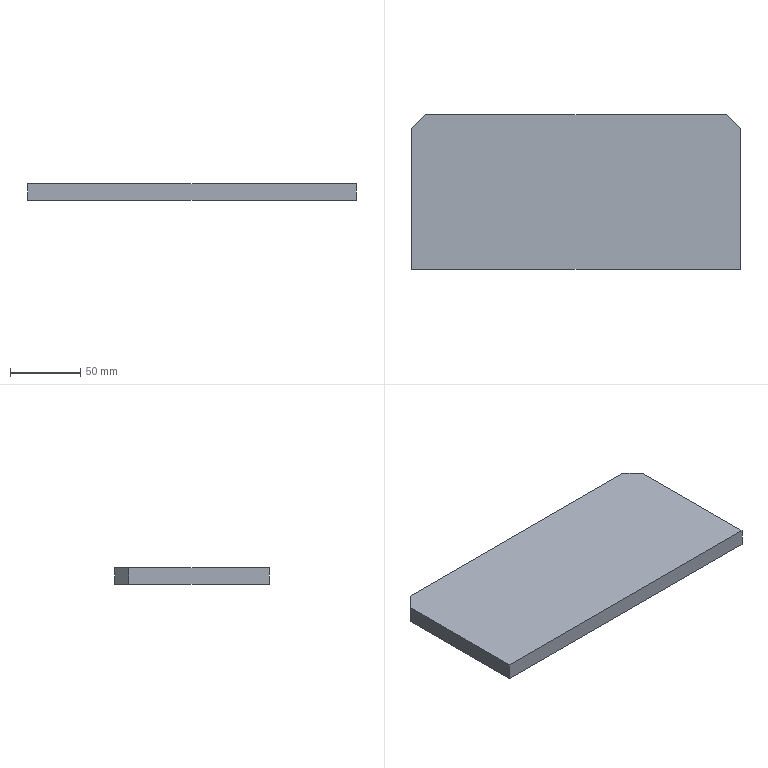Part | SolidWorks | features BaseBody 1 | 1 solid | 8 faces | box 234 x 110 x 12 mm | volume 307680 mm3 | plane 8
STEP:
#1=CARTESIAN_POINT('',(117.,-55.,0.));
#2=VERTEX_POINT('',#1);
#3=CARTESIAN_POINT('',(117.,45.,0.));
#4=VERTEX_POINT('',#3);
#5=CARTESIAN_POINT('',(117.,45.,0.));
#6=DIRECTION('',(0.,1.,0.));
#7=VECTOR('',#6,1000.);
#8=LINE('',#5,#7);
#9=EDGE_CURVE('',#2,#4,#8,.T.);
#10=ORIENTED_EDGE('',*,*,#9,.T.);
#11=CARTESIAN_POINT('',(117.,45.,12.));
#12=VERTEX_POINT('',#11);
#13=CARTESIAN_POINT('',(117.,45.,12.));
#14=DIRECTION('',(0.,0.,-1.));
#15=VECTOR('',#14,1000.);
#16=LINE('',#13,#15);
#17=EDGE_CURVE('',#12,#4,#16,.T.);
#18=ORIENTED_EDGE('',*,*,#17,.F.);
#19=CARTESIAN_POINT('',(117.,-55.,12.));
#20=VERTEX_POINT('',#19);
#21=CARTESIAN_POINT('',(117.,45.,12.));
#22=DIRECTION('',(0.,1.,0.));
#23=VECTOR('',#22,1000.);
#24=LINE('',#21,#23);
#25=EDGE_CURVE('',#20,#12,#24,.T.);
#26=ORIENTED_EDGE('',*,*,#25,.F.);
#27=CARTESIAN_POINT('',(117.,-55.,12.));
#28=DIRECTION('',(0.,0.,-1.));
#29=VECTOR('',#28,1000.);
#30=LINE('',#27,#29);
#31=EDGE_CURVE('',#20,#2,#30,.T.);
#32=ORIENTED_EDGE('',*,*,#31,.T.);
#33=EDGE_LOOP('',(#10,#18,#26,#32));
#34=FACE_OUTER_BOUND('',#33,.T.);
#35=CARTESIAN_POINT('',(117.,45.,12.));
#36=DIRECTION('',(-1.,0.,0.));
#37=DIRECTION('',(0.,0.,1.));
#38=AXIS2_PLACEMENT_3D('',#35,#36,#37);
#39=PLANE('',#38);
#40=ADVANCED_FACE('',(#34),#39,.F.);
#41=CARTESIAN_POINT('',(107.,55.,0.));
#42=VERTEX_POINT('',#41);
#43=CARTESIAN_POINT('',(107.,55.,0.));
#44=DIRECTION('',(-0.7071,0.7071,0.));
#45=VECTOR('',#44,1000.);
#46=LINE('',#43,#45);
#47=EDGE_CURVE('',#4,#42,#46,.T.);
#48=ORIENTED_EDGE('',*,*,#47,.T.);
#49=CARTESIAN_POINT('',(107.,55.,12.));
#50=VERTEX_POINT('',#49);
#51=CARTESIAN_POINT('',(107.,55.,12.));
#52=DIRECTION('',(0.,0.,-1.));
#53=VECTOR('',#52,1000.);
#54=LINE('',#51,#53);
#55=EDGE_CURVE('',#50,#42,#54,.T.);
#56=ORIENTED_EDGE('',*,*,#55,.F.);
#57=CARTESIAN_POINT('',(107.,55.,12.));
#58=DIRECTION('',(-0.7071,0.7071,0.));
#59=VECTOR('',#58,1000.);
#60=LINE('',#57,#59);
#61=EDGE_CURVE('',#12,#50,#60,.T.);
#62=ORIENTED_EDGE('',*,*,#61,.F.);
#63=ORIENTED_EDGE('',*,*,#17,.T.);
#64=EDGE_LOOP('',(#48,#56,#62,#63));
#65=FACE_OUTER_BOUND('',#64,.T.);
#66=CARTESIAN_POINT('',(107.,55.,12.));
#67=DIRECTION('',(-0.7071,-0.7071,0.));
#68=DIRECTION('',(0.7071,-0.7071,0.));
#69=AXIS2_PLACEMENT_3D('',#66,#67,#68);
#70=PLANE('',#69);
#71=ADVANCED_FACE('',(#65),#70,.F.);
#72=CARTESIAN_POINT('',(-107.,55.,0.));
#73=VERTEX_POINT('',#72);
#74=CARTESIAN_POINT('',(-107.,55.,0.));
#75=DIRECTION('',(-1.,0.,0.));
#76=VECTOR('',#75,1000.);
#77=LINE('',#74,#76);
#78=EDGE_CURVE('',#42,#73,#77,.T.);
#79=ORIENTED_EDGE('',*,*,#78,.T.);
#80=CARTESIAN_POINT('',(-107.,55.,12.));
#81=VERTEX_POINT('',#80);
#82=CARTESIAN_POINT('',(-107.,55.,12.));
#83=DIRECTION('',(0.,0.,-1.));
#84=VECTOR('',#83,1000.);
#85=LINE('',#82,#84);
#86=EDGE_CURVE('',#81,#73,#85,.T.);
#87=ORIENTED_EDGE('',*,*,#86,.F.);
#88=CARTESIAN_POINT('',(-107.,55.,12.));
#89=DIRECTION('',(-1.,0.,0.));
#90=VECTOR('',#89,1000.);
#91=LINE('',#88,#90);
#92=EDGE_CURVE('',#50,#81,#91,.T.);
#93=ORIENTED_EDGE('',*,*,#92,.F.);
#94=ORIENTED_EDGE('',*,*,#55,.T.);
#95=EDGE_LOOP('',(#79,#87,#93,#94));
#96=FACE_OUTER_BOUND('',#95,.T.);
#97=CARTESIAN_POINT('',(-107.,55.,12.));
#98=DIRECTION('',(0.,-1.,0.));
#99=DIRECTION('',(0.,0.,-1.));
#100=AXIS2_PLACEMENT_3D('',#97,#98,#99);
#101=PLANE('',#100);
#102=ADVANCED_FACE('',(#96),#101,.F.);
#103=CARTESIAN_POINT('',(-117.,45.,0.));
#104=VERTEX_POINT('',#103);
#105=CARTESIAN_POINT('',(-117.,45.,0.));
#106=DIRECTION('',(-0.7071,-0.7071,0.));
#107=VECTOR('',#106,1000.);
#108=LINE('',#105,#107);
#109=EDGE_CURVE('',#73,#104,#108,.T.);
#110=ORIENTED_EDGE('',*,*,#109,.T.);
#111=CARTESIAN_POINT('',(-117.,45.,12.));
#112=VERTEX_POINT('',#111);
#113=CARTESIAN_POINT('',(-117.,45.,12.));
#114=DIRECTION('',(0.,0.,-1.));
#115=VECTOR('',#114,1000.);
#116=LINE('',#113,#115);
#117=EDGE_CURVE('',#112,#104,#116,.T.);
#118=ORIENTED_EDGE('',*,*,#117,.F.);
#119=CARTESIAN_POINT('',(-117.,45.,12.));
#120=DIRECTION('',(-0.7071,-0.7071,0.));
#121=VECTOR('',#120,1000.);
#122=LINE('',#119,#121);
#123=EDGE_CURVE('',#81,#112,#122,.T.);
#124=ORIENTED_EDGE('',*,*,#123,.F.);
#125=ORIENTED_EDGE('',*,*,#86,.T.);
#126=EDGE_LOOP('',(#110,#118,#124,#125));
#127=FACE_OUTER_BOUND('',#126,.T.);
#128=CARTESIAN_POINT('',(-117.,45.,12.));
#129=DIRECTION('',(0.7071,-0.7071,0.));
#130=DIRECTION('',(0.7071,0.7071,0.));
#131=AXIS2_PLACEMENT_3D('',#128,#129,#130);
#132=PLANE('',#131);
#133=ADVANCED_FACE('',(#127),#132,.F.);
#134=CARTESIAN_POINT('',(-117.,-55.,0.));
#135=VERTEX_POINT('',#134);
#136=CARTESIAN_POINT('',(-117.,45.,0.));
#137=DIRECTION('',(0.,-1.,0.));
#138=VECTOR('',#137,1000.);
#139=LINE('',#136,#138);
#140=EDGE_CURVE('',#104,#135,#139,.T.);
#141=ORIENTED_EDGE('',*,*,#140,.T.);
#142=CARTESIAN_POINT('',(-117.,-55.,12.));
#143=VERTEX_POINT('',#142);
#144=CARTESIAN_POINT('',(-117.,-55.,12.));
#145=DIRECTION('',(0.,0.,-1.));
#146=VECTOR('',#145,1000.);
#147=LINE('',#144,#146);
#148=EDGE_CURVE('',#143,#135,#147,.T.);
#149=ORIENTED_EDGE('',*,*,#148,.F.);
#150=CARTESIAN_POINT('',(-117.,45.,12.));
#151=DIRECTION('',(0.,-1.,0.));
#152=VECTOR('',#151,1000.);
#153=LINE('',#150,#152);
#154=EDGE_CURVE('',#112,#143,#153,.T.);
#155=ORIENTED_EDGE('',*,*,#154,.F.);
#156=ORIENTED_EDGE('',*,*,#117,.T.);
#157=EDGE_LOOP('',(#141,#149,#155,#156));
#158=FACE_OUTER_BOUND('',#157,.T.);
#159=CARTESIAN_POINT('',(-117.,45.,12.));
#160=DIRECTION('',(1.,0.,0.));
#161=DIRECTION('',(0.,1.,0.));
#162=AXIS2_PLACEMENT_3D('',#159,#160,#161);
#163=PLANE('',#162);
#164=ADVANCED_FACE('',(#158),#163,.F.);
#165=CARTESIAN_POINT('',(-117.,-55.,0.));
#166=DIRECTION('',(1.,0.,0.));
#167=VECTOR('',#166,1000.);
#168=LINE('',#165,#167);
#169=EDGE_CURVE('',#135,#2,#168,.T.);
#170=ORIENTED_EDGE('',*,*,#169,.T.);
#171=ORIENTED_EDGE('',*,*,#31,.F.);
#172=CARTESIAN_POINT('',(-117.,-55.,12.));
#173=DIRECTION('',(1.,0.,0.));
#174=VECTOR('',#173,1000.);
#175=LINE('',#172,#174);
#176=EDGE_CURVE('',#143,#20,#175,.T.);
#177=ORIENTED_EDGE('',*,*,#176,.F.);
#178=ORIENTED_EDGE('',*,*,#148,.T.);
#179=EDGE_LOOP('',(#170,#171,#177,#178));
#180=FACE_OUTER_BOUND('',#179,.T.);
#181=CARTESIAN_POINT('',(-117.,-55.,12.));
#182=DIRECTION('',(0.,1.,0.));
#183=DIRECTION('',(0.,0.,1.));
#184=AXIS2_PLACEMENT_3D('',#181,#182,#183);
#185=PLANE('',#184);
#186=ADVANCED_FACE('',(#180),#185,.F.);
#187=ORIENTED_EDGE('',*,*,#25,.T.);
#188=ORIENTED_EDGE('',*,*,#61,.T.);
#189=ORIENTED_EDGE('',*,*,#92,.T.);
#190=ORIENTED_EDGE('',*,*,#123,.T.);
#191=ORIENTED_EDGE('',*,*,#154,.T.);
#192=ORIENTED_EDGE('',*,*,#176,.T.);
#193=EDGE_LOOP('',(#187,#188,#189,#190,#191,#192));
#194=FACE_OUTER_BOUND('',#193,.T.);
#195=CARTESIAN_POINT('',(0.,0.,12.));
#196=DIRECTION('',(0.,0.,1.));
#197=DIRECTION('',(1.,0.,0.));
#198=AXIS2_PLACEMENT_3D('',#195,#196,#197);
#199=PLANE('',#198);
#200=ADVANCED_FACE('',(#194),#199,.T.);
#201=ORIENTED_EDGE('',*,*,#9,.F.);
#202=ORIENTED_EDGE('',*,*,#169,.F.);
#203=ORIENTED_EDGE('',*,*,#140,.F.);
#204=ORIENTED_EDGE('',*,*,#109,.F.);
#205=ORIENTED_EDGE('',*,*,#78,.F.);
#206=ORIENTED_EDGE('',*,*,#47,.F.);
#207=EDGE_LOOP('',(#201,#202,#203,#204,#205,#206));
#208=FACE_OUTER_BOUND('',#207,.T.);
#209=CARTESIAN_POINT('',(0.,0.,0.));
#210=DIRECTION('',(0.,0.,1.));
#211=DIRECTION('',(1.,0.,0.));
#212=AXIS2_PLACEMENT_3D('',#209,#210,#211);
#213=PLANE('',#212);
#214=ADVANCED_FACE('',(#208),#213,.F.);
#215=CLOSED_SHELL('',(#40,#71,#102,#133,#164,#186,#200,#214));
#216=MANIFOLD_SOLID_BREP('',#215);
#217=CARTESIAN_POINT('',(0.,0.,0.));
#218=DIRECTION('',(0.,0.,1.));
#219=DIRECTION('',(1.,0.,0.));
#220=AXIS2_PLACEMENT_3D('',#217,#218,#219);
#221=(LENGTH_UNIT()NAMED_UNIT(*)SI_UNIT(.MILLI.,.METRE.));
#222=UNCERTAINTY_MEASURE_WITH_UNIT(LENGTH_MEASURE(0.00001),#221,'','');
#223=(NAMED_UNIT(*)PLANE_ANGLE_UNIT()SI_UNIT($,.RADIAN.));
#224=(NAMED_UNIT(*)SI_UNIT($,.STERADIAN.)SOLID_ANGLE_UNIT());
#225=(GEOMETRIC_REPRESENTATION_CONTEXT(3)GLOBAL_UNCERTAINTY_ASSIGNED_CONTEXT((#222))GLOBAL_UNIT_ASSIGNED_CONTEXT((#221,#223,#224))REPRESENTATION_CONTEXT('',''));
#226=ADVANCED_BREP_SHAPE_REPRESENTATION('',(#216,#220),#225);